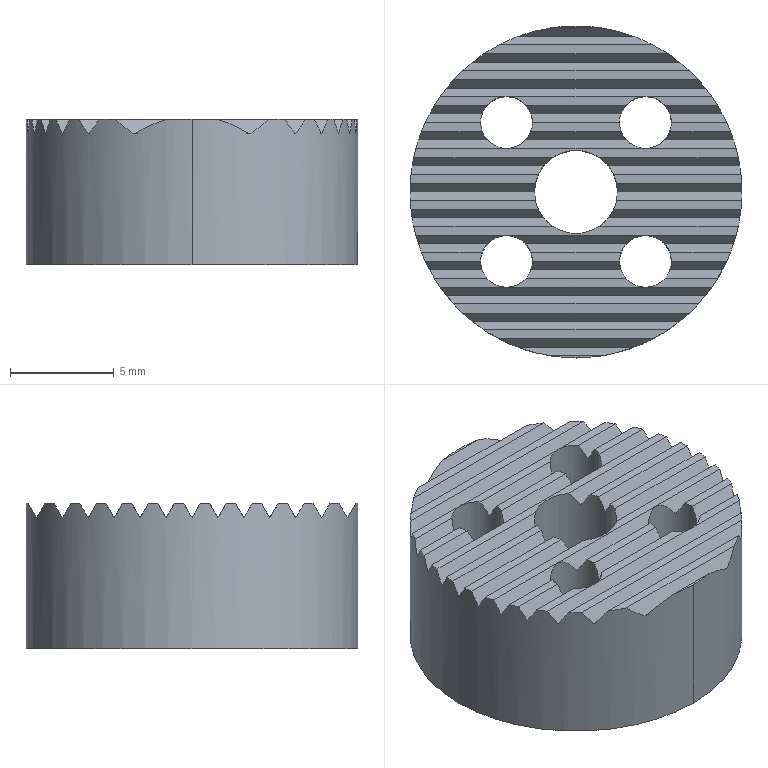Part | 1 solid | 81 faces | box 16 x 16 x 7 mm | volume 1144 mm3 | plane 69 | cylinder 12 | commonest cylinder face diameters 2.5 x8 4 x2 16 x2